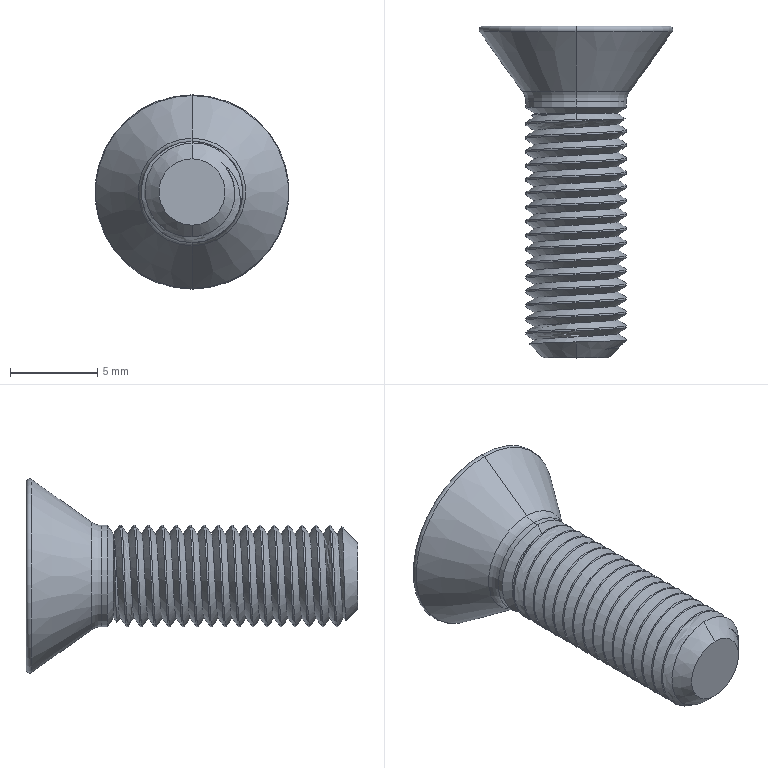Part | STEP file | Screw M6 - 15mm flat head | 1 solid | 58 faces | box 11.124 x 19 x 11.124 mm | volume 537.747 mm3 | cylinder 35 | plane 9 | cone 8 | torus 4 | spline 2 | commonest cylinder face diameters 5.8 x35